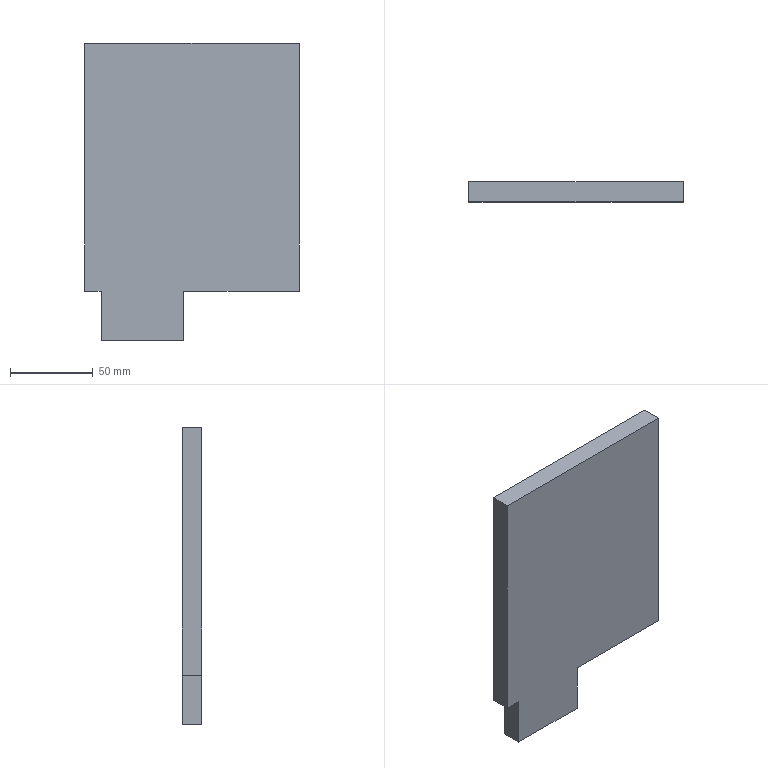Part | SolidWorks | features Extrusion 1 | 1 solid | 10 faces | box 130 x 12 x 180 mm | volume 252000 mm3 | plane 10
STEP:
#1=CARTESIAN_POINT('',(0.,0.,-150.));
#2=VERTEX_POINT('',#1);
#3=CARTESIAN_POINT('',(0.,0.,0.));
#4=VERTEX_POINT('',#3);
#5=CARTESIAN_POINT('',(0.,0.,-150.));
#6=DIRECTION('',(0.,0.,1.));
#7=VECTOR('',#6,1000.);
#8=LINE('',#5,#7);
#9=EDGE_CURVE('',#2,#4,#8,.T.);
#10=ORIENTED_EDGE('',*,*,#9,.T.);
#11=CARTESIAN_POINT('',(0.,12.,0.));
#12=VERTEX_POINT('',#11);
#13=CARTESIAN_POINT('',(0.,12.,0.));
#14=DIRECTION('',(0.,-1.,0.));
#15=VECTOR('',#14,1000.);
#16=LINE('',#13,#15);
#17=EDGE_CURVE('',#12,#4,#16,.T.);
#18=ORIENTED_EDGE('',*,*,#17,.F.);
#19=CARTESIAN_POINT('',(0.,12.,-150.));
#20=VERTEX_POINT('',#19);
#21=CARTESIAN_POINT('',(0.,12.,-150.));
#22=DIRECTION('',(0.,0.,1.));
#23=VECTOR('',#22,1000.);
#24=LINE('',#21,#23);
#25=EDGE_CURVE('',#20,#12,#24,.T.);
#26=ORIENTED_EDGE('',*,*,#25,.F.);
#27=CARTESIAN_POINT('',(0.,12.,-150.));
#28=DIRECTION('',(0.,-1.,0.));
#29=VECTOR('',#28,1000.);
#30=LINE('',#27,#29);
#31=EDGE_CURVE('',#20,#2,#30,.T.);
#32=ORIENTED_EDGE('',*,*,#31,.T.);
#33=EDGE_LOOP('',(#10,#18,#26,#32));
#34=FACE_OUTER_BOUND('',#33,.T.);
#35=CARTESIAN_POINT('',(0.,12.,-150.));
#36=DIRECTION('',(1.,0.,0.));
#37=DIRECTION('',(0.,0.,-1.));
#38=AXIS2_PLACEMENT_3D('',#35,#36,#37);
#39=PLANE('',#38);
#40=ADVANCED_FACE('',(#34),#39,.F.);
#41=CARTESIAN_POINT('',(130.,0.,0.));
#42=VERTEX_POINT('',#41);
#43=CARTESIAN_POINT('',(0.,0.,0.));
#44=DIRECTION('',(1.,0.,0.));
#45=VECTOR('',#44,1000.);
#46=LINE('',#43,#45);
#47=EDGE_CURVE('',#4,#42,#46,.T.);
#48=ORIENTED_EDGE('',*,*,#47,.T.);
#49=CARTESIAN_POINT('',(130.,12.,0.));
#50=VERTEX_POINT('',#49);
#51=CARTESIAN_POINT('',(130.,12.,0.));
#52=DIRECTION('',(0.,-1.,0.));
#53=VECTOR('',#52,1000.);
#54=LINE('',#51,#53);
#55=EDGE_CURVE('',#50,#42,#54,.T.);
#56=ORIENTED_EDGE('',*,*,#55,.F.);
#57=CARTESIAN_POINT('',(0.,12.,0.));
#58=DIRECTION('',(1.,0.,0.));
#59=VECTOR('',#58,1000.);
#60=LINE('',#57,#59);
#61=EDGE_CURVE('',#12,#50,#60,.T.);
#62=ORIENTED_EDGE('',*,*,#61,.F.);
#63=ORIENTED_EDGE('',*,*,#17,.T.);
#64=EDGE_LOOP('',(#48,#56,#62,#63));
#65=FACE_OUTER_BOUND('',#64,.T.);
#66=CARTESIAN_POINT('',(0.,12.,0.));
#67=DIRECTION('',(0.,0.,-1.));
#68=DIRECTION('',(-1.,0.,0.));
#69=AXIS2_PLACEMENT_3D('',#66,#67,#68);
#70=PLANE('',#69);
#71=ADVANCED_FACE('',(#65),#70,.F.);
#72=CARTESIAN_POINT('',(130.,0.,-150.));
#73=VERTEX_POINT('',#72);
#74=CARTESIAN_POINT('',(130.,0.,0.));
#75=DIRECTION('',(0.,0.,-1.));
#76=VECTOR('',#75,1000.);
#77=LINE('',#74,#76);
#78=EDGE_CURVE('',#42,#73,#77,.T.);
#79=ORIENTED_EDGE('',*,*,#78,.T.);
#80=CARTESIAN_POINT('',(130.,12.,-150.));
#81=VERTEX_POINT('',#80);
#82=CARTESIAN_POINT('',(130.,12.,-150.));
#83=DIRECTION('',(0.,-1.,0.));
#84=VECTOR('',#83,1000.);
#85=LINE('',#82,#84);
#86=EDGE_CURVE('',#81,#73,#85,.T.);
#87=ORIENTED_EDGE('',*,*,#86,.F.);
#88=CARTESIAN_POINT('',(130.,12.,0.));
#89=DIRECTION('',(0.,0.,-1.));
#90=VECTOR('',#89,1000.);
#91=LINE('',#88,#90);
#92=EDGE_CURVE('',#50,#81,#91,.T.);
#93=ORIENTED_EDGE('',*,*,#92,.F.);
#94=ORIENTED_EDGE('',*,*,#55,.T.);
#95=EDGE_LOOP('',(#79,#87,#93,#94));
#96=FACE_OUTER_BOUND('',#95,.T.);
#97=CARTESIAN_POINT('',(130.,12.,0.));
#98=DIRECTION('',(-1.,0.,0.));
#99=DIRECTION('',(0.,0.,1.));
#100=AXIS2_PLACEMENT_3D('',#97,#98,#99);
#101=PLANE('',#100);
#102=ADVANCED_FACE('',(#96),#101,.F.);
#103=CARTESIAN_POINT('',(60.,0.,-150.));
#104=VERTEX_POINT('',#103);
#105=CARTESIAN_POINT('',(130.,0.,-150.));
#106=DIRECTION('',(-1.,0.,0.));
#107=VECTOR('',#106,1000.);
#108=LINE('',#105,#107);
#109=EDGE_CURVE('',#73,#104,#108,.T.);
#110=ORIENTED_EDGE('',*,*,#109,.T.);
#111=CARTESIAN_POINT('',(60.,12.,-150.));
#112=VERTEX_POINT('',#111);
#113=CARTESIAN_POINT('',(60.,12.,-150.));
#114=DIRECTION('',(0.,-1.,0.));
#115=VECTOR('',#114,1000.);
#116=LINE('',#113,#115);
#117=EDGE_CURVE('',#112,#104,#116,.T.);
#118=ORIENTED_EDGE('',*,*,#117,.F.);
#119=CARTESIAN_POINT('',(130.,12.,-150.));
#120=DIRECTION('',(-1.,0.,0.));
#121=VECTOR('',#120,1000.);
#122=LINE('',#119,#121);
#123=EDGE_CURVE('',#81,#112,#122,.T.);
#124=ORIENTED_EDGE('',*,*,#123,.F.);
#125=ORIENTED_EDGE('',*,*,#86,.T.);
#126=EDGE_LOOP('',(#110,#118,#124,#125));
#127=FACE_OUTER_BOUND('',#126,.T.);
#128=CARTESIAN_POINT('',(130.,12.,-150.));
#129=DIRECTION('',(0.,0.,1.));
#130=DIRECTION('',(1.,0.,0.));
#131=AXIS2_PLACEMENT_3D('',#128,#129,#130);
#132=PLANE('',#131);
#133=ADVANCED_FACE('',(#127),#132,.F.);
#134=CARTESIAN_POINT('',(60.,0.,-180.));
#135=VERTEX_POINT('',#134);
#136=CARTESIAN_POINT('',(60.,0.,-150.));
#137=DIRECTION('',(0.,0.,-1.));
#138=VECTOR('',#137,1000.);
#139=LINE('',#136,#138);
#140=EDGE_CURVE('',#104,#135,#139,.T.);
#141=ORIENTED_EDGE('',*,*,#140,.T.);
#142=CARTESIAN_POINT('',(60.,12.,-180.));
#143=VERTEX_POINT('',#142);
#144=CARTESIAN_POINT('',(60.,12.,-180.));
#145=DIRECTION('',(0.,-1.,0.));
#146=VECTOR('',#145,1000.);
#147=LINE('',#144,#146);
#148=EDGE_CURVE('',#143,#135,#147,.T.);
#149=ORIENTED_EDGE('',*,*,#148,.F.);
#150=CARTESIAN_POINT('',(60.,12.,-150.));
#151=DIRECTION('',(0.,0.,-1.));
#152=VECTOR('',#151,1000.);
#153=LINE('',#150,#152);
#154=EDGE_CURVE('',#112,#143,#153,.T.);
#155=ORIENTED_EDGE('',*,*,#154,.F.);
#156=ORIENTED_EDGE('',*,*,#117,.T.);
#157=EDGE_LOOP('',(#141,#149,#155,#156));
#158=FACE_OUTER_BOUND('',#157,.T.);
#159=CARTESIAN_POINT('',(60.,12.,-150.));
#160=DIRECTION('',(-1.,0.,0.));
#161=DIRECTION('',(0.,0.,1.));
#162=AXIS2_PLACEMENT_3D('',#159,#160,#161);
#163=PLANE('',#162);
#164=ADVANCED_FACE('',(#158),#163,.F.);
#165=CARTESIAN_POINT('',(10.,0.,-180.));
#166=VERTEX_POINT('',#165);
#167=CARTESIAN_POINT('',(60.,0.,-180.));
#168=DIRECTION('',(-1.,0.,0.));
#169=VECTOR('',#168,1000.);
#170=LINE('',#167,#169);
#171=EDGE_CURVE('',#135,#166,#170,.T.);
#172=ORIENTED_EDGE('',*,*,#171,.T.);
#173=CARTESIAN_POINT('',(10.,12.,-180.));
#174=VERTEX_POINT('',#173);
#175=CARTESIAN_POINT('',(10.,12.,-180.));
#176=DIRECTION('',(0.,-1.,0.));
#177=VECTOR('',#176,1000.);
#178=LINE('',#175,#177);
#179=EDGE_CURVE('',#174,#166,#178,.T.);
#180=ORIENTED_EDGE('',*,*,#179,.F.);
#181=CARTESIAN_POINT('',(60.,12.,-180.));
#182=DIRECTION('',(-1.,0.,0.));
#183=VECTOR('',#182,1000.);
#184=LINE('',#181,#183);
#185=EDGE_CURVE('',#143,#174,#184,.T.);
#186=ORIENTED_EDGE('',*,*,#185,.F.);
#187=ORIENTED_EDGE('',*,*,#148,.T.);
#188=EDGE_LOOP('',(#172,#180,#186,#187));
#189=FACE_OUTER_BOUND('',#188,.T.);
#190=CARTESIAN_POINT('',(60.,12.,-180.));
#191=DIRECTION('',(0.,0.,1.));
#192=DIRECTION('',(1.,0.,0.));
#193=AXIS2_PLACEMENT_3D('',#190,#191,#192);
#194=PLANE('',#193);
#195=ADVANCED_FACE('',(#189),#194,.F.);
#196=CARTESIAN_POINT('',(10.,0.,-150.));
#197=VERTEX_POINT('',#196);
#198=CARTESIAN_POINT('',(10.,0.,-180.));
#199=DIRECTION('',(0.,0.,1.));
#200=VECTOR('',#199,1000.);
#201=LINE('',#198,#200);
#202=EDGE_CURVE('',#166,#197,#201,.T.);
#203=ORIENTED_EDGE('',*,*,#202,.T.);
#204=CARTESIAN_POINT('',(10.,12.,-150.));
#205=VERTEX_POINT('',#204);
#206=CARTESIAN_POINT('',(10.,12.,-150.));
#207=DIRECTION('',(0.,-1.,0.));
#208=VECTOR('',#207,1000.);
#209=LINE('',#206,#208);
#210=EDGE_CURVE('',#205,#197,#209,.T.);
#211=ORIENTED_EDGE('',*,*,#210,.F.);
#212=CARTESIAN_POINT('',(10.,12.,-180.));
#213=DIRECTION('',(0.,0.,1.));
#214=VECTOR('',#213,1000.);
#215=LINE('',#212,#214);
#216=EDGE_CURVE('',#174,#205,#215,.T.);
#217=ORIENTED_EDGE('',*,*,#216,.F.);
#218=ORIENTED_EDGE('',*,*,#179,.T.);
#219=EDGE_LOOP('',(#203,#211,#217,#218));
#220=FACE_OUTER_BOUND('',#219,.T.);
#221=CARTESIAN_POINT('',(10.,12.,-180.));
#222=DIRECTION('',(1.,0.,0.));
#223=DIRECTION('',(0.,0.,-1.));
#224=AXIS2_PLACEMENT_3D('',#221,#222,#223);
#225=PLANE('',#224);
#226=ADVANCED_FACE('',(#220),#225,.F.);
#227=CARTESIAN_POINT('',(10.,0.,-150.));
#228=DIRECTION('',(-1.,0.,0.));
#229=VECTOR('',#228,1000.);
#230=LINE('',#227,#229);
#231=EDGE_CURVE('',#197,#2,#230,.T.);
#232=ORIENTED_EDGE('',*,*,#231,.T.);
#233=ORIENTED_EDGE('',*,*,#31,.F.);
#234=CARTESIAN_POINT('',(10.,12.,-150.));
#235=DIRECTION('',(-1.,0.,0.));
#236=VECTOR('',#235,1000.);
#237=LINE('',#234,#236);
#238=EDGE_CURVE('',#205,#20,#237,.T.);
#239=ORIENTED_EDGE('',*,*,#238,.F.);
#240=ORIENTED_EDGE('',*,*,#210,.T.);
#241=EDGE_LOOP('',(#232,#233,#239,#240));
#242=FACE_OUTER_BOUND('',#241,.T.);
#243=CARTESIAN_POINT('',(10.,12.,-150.));
#244=DIRECTION('',(0.,0.,1.));
#245=DIRECTION('',(1.,0.,0.));
#246=AXIS2_PLACEMENT_3D('',#243,#244,#245);
#247=PLANE('',#246);
#248=ADVANCED_FACE('',(#242),#247,.F.);
#249=ORIENTED_EDGE('',*,*,#25,.T.);
#250=ORIENTED_EDGE('',*,*,#61,.T.);
#251=ORIENTED_EDGE('',*,*,#92,.T.);
#252=ORIENTED_EDGE('',*,*,#123,.T.);
#253=ORIENTED_EDGE('',*,*,#154,.T.);
#254=ORIENTED_EDGE('',*,*,#185,.T.);
#255=ORIENTED_EDGE('',*,*,#216,.T.);
#256=ORIENTED_EDGE('',*,*,#238,.T.);
#257=EDGE_LOOP('',(#249,#250,#251,#252,#253,#254,#255,#256));
#258=FACE_OUTER_BOUND('',#257,.T.);
#259=CARTESIAN_POINT('',(0.,12.,0.));
#260=DIRECTION('',(0.,1.,0.));
#261=DIRECTION('',(0.,0.,1.));
#262=AXIS2_PLACEMENT_3D('',#259,#260,#261);
#263=PLANE('',#262);
#264=ADVANCED_FACE('',(#258),#263,.T.);
#265=ORIENTED_EDGE('',*,*,#9,.F.);
#266=ORIENTED_EDGE('',*,*,#231,.F.);
#267=ORIENTED_EDGE('',*,*,#202,.F.);
#268=ORIENTED_EDGE('',*,*,#171,.F.);
#269=ORIENTED_EDGE('',*,*,#140,.F.);
#270=ORIENTED_EDGE('',*,*,#109,.F.);
#271=ORIENTED_EDGE('',*,*,#78,.F.);
#272=ORIENTED_EDGE('',*,*,#47,.F.);
#273=EDGE_LOOP('',(#265,#266,#267,#268,#269,#270,#271,#272));
#274=FACE_OUTER_BOUND('',#273,.T.);
#275=CARTESIAN_POINT('',(0.,0.,0.));
#276=DIRECTION('',(0.,1.,0.));
#277=DIRECTION('',(0.,0.,1.));
#278=AXIS2_PLACEMENT_3D('',#275,#276,#277);
#279=PLANE('',#278);
#280=ADVANCED_FACE('',(#274),#279,.F.);
#281=CLOSED_SHELL('',(#40,#71,#102,#133,#164,#195,#226,#248,#264,#280));
#282=MANIFOLD_SOLID_BREP('',#281);
#283=CARTESIAN_POINT('',(0.,0.,0.));
#284=DIRECTION('',(0.,0.,1.));
#285=DIRECTION('',(1.,0.,0.));
#286=AXIS2_PLACEMENT_3D('',#283,#284,#285);
#287=(LENGTH_UNIT()NAMED_UNIT(*)SI_UNIT(.MILLI.,.METRE.));
#288=UNCERTAINTY_MEASURE_WITH_UNIT(LENGTH_MEASURE(0.00001),#287,'','');
#289=(NAMED_UNIT(*)PLANE_ANGLE_UNIT()SI_UNIT($,.RADIAN.));
#290=(NAMED_UNIT(*)SI_UNIT($,.STERADIAN.)SOLID_ANGLE_UNIT());
#291=(GEOMETRIC_REPRESENTATION_CONTEXT(3)GLOBAL_UNCERTAINTY_ASSIGNED_CONTEXT((#288))GLOBAL_UNIT_ASSIGNED_CONTEXT((#287,#289,#290))REPRESENTATION_CONTEXT('',''));
#292=ADVANCED_BREP_SHAPE_REPRESENTATION('',(#282,#286),#291);